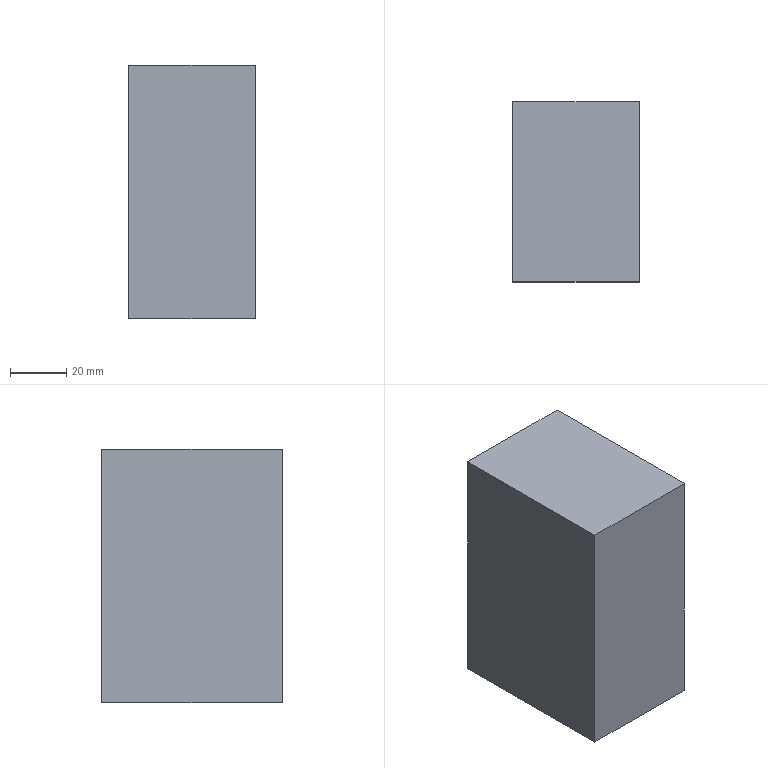Part | SolidWorks | features Extrusion 1 | 1 solid | 6 faces | box 45 x 64 x 90 mm | volume 259200 mm3 | plane 6
STEP:
#1=CARTESIAN_POINT('',(22.5,0.,45.));
#2=VERTEX_POINT('',#1);
#3=CARTESIAN_POINT('',(22.5,0.,-45.));
#4=VERTEX_POINT('',#3);
#5=CARTESIAN_POINT('',(22.5,0.,45.));
#6=DIRECTION('',(0.,0.,-1.));
#7=VECTOR('',#6,1000.);
#8=LINE('',#5,#7);
#9=EDGE_CURVE('',#2,#4,#8,.T.);
#10=ORIENTED_EDGE('',*,*,#9,.T.);
#11=CARTESIAN_POINT('',(22.5,64.,-45.));
#12=VERTEX_POINT('',#11);
#13=CARTESIAN_POINT('',(22.5,64.,-45.));
#14=DIRECTION('',(0.,-1.,0.));
#15=VECTOR('',#14,1000.);
#16=LINE('',#13,#15);
#17=EDGE_CURVE('',#12,#4,#16,.T.);
#18=ORIENTED_EDGE('',*,*,#17,.F.);
#19=CARTESIAN_POINT('',(22.5,64.,45.));
#20=VERTEX_POINT('',#19);
#21=CARTESIAN_POINT('',(22.5,64.,45.));
#22=DIRECTION('',(0.,0.,-1.));
#23=VECTOR('',#22,1000.);
#24=LINE('',#21,#23);
#25=EDGE_CURVE('',#20,#12,#24,.T.);
#26=ORIENTED_EDGE('',*,*,#25,.F.);
#27=CARTESIAN_POINT('',(22.5,64.,45.));
#28=DIRECTION('',(0.,-1.,0.));
#29=VECTOR('',#28,1000.);
#30=LINE('',#27,#29);
#31=EDGE_CURVE('',#20,#2,#30,.T.);
#32=ORIENTED_EDGE('',*,*,#31,.T.);
#33=EDGE_LOOP('',(#10,#18,#26,#32));
#34=FACE_OUTER_BOUND('',#33,.T.);
#35=CARTESIAN_POINT('',(22.5,64.,45.));
#36=DIRECTION('',(-1.,0.,0.));
#37=DIRECTION('',(0.,0.,1.));
#38=AXIS2_PLACEMENT_3D('',#35,#36,#37);
#39=PLANE('',#38);
#40=ADVANCED_FACE('',(#34),#39,.F.);
#41=CARTESIAN_POINT('',(-22.5,0.,-45.));
#42=VERTEX_POINT('',#41);
#43=CARTESIAN_POINT('',(-22.5,0.,-45.));
#44=DIRECTION('',(-1.,0.,0.));
#45=VECTOR('',#44,1000.);
#46=LINE('',#43,#45);
#47=EDGE_CURVE('',#4,#42,#46,.T.);
#48=ORIENTED_EDGE('',*,*,#47,.T.);
#49=CARTESIAN_POINT('',(-22.5,64.,-45.));
#50=VERTEX_POINT('',#49);
#51=CARTESIAN_POINT('',(-22.5,64.,-45.));
#52=DIRECTION('',(0.,-1.,0.));
#53=VECTOR('',#52,1000.);
#54=LINE('',#51,#53);
#55=EDGE_CURVE('',#50,#42,#54,.T.);
#56=ORIENTED_EDGE('',*,*,#55,.F.);
#57=CARTESIAN_POINT('',(-22.5,64.,-45.));
#58=DIRECTION('',(-1.,0.,0.));
#59=VECTOR('',#58,1000.);
#60=LINE('',#57,#59);
#61=EDGE_CURVE('',#12,#50,#60,.T.);
#62=ORIENTED_EDGE('',*,*,#61,.F.);
#63=ORIENTED_EDGE('',*,*,#17,.T.);
#64=EDGE_LOOP('',(#48,#56,#62,#63));
#65=FACE_OUTER_BOUND('',#64,.T.);
#66=CARTESIAN_POINT('',(-22.5,64.,-45.));
#67=DIRECTION('',(0.,0.,1.));
#68=DIRECTION('',(1.,0.,0.));
#69=AXIS2_PLACEMENT_3D('',#66,#67,#68);
#70=PLANE('',#69);
#71=ADVANCED_FACE('',(#65),#70,.F.);
#72=CARTESIAN_POINT('',(-22.5,0.,45.));
#73=VERTEX_POINT('',#72);
#74=CARTESIAN_POINT('',(-22.5,0.,45.));
#75=DIRECTION('',(0.,0.,1.));
#76=VECTOR('',#75,1000.);
#77=LINE('',#74,#76);
#78=EDGE_CURVE('',#42,#73,#77,.T.);
#79=ORIENTED_EDGE('',*,*,#78,.T.);
#80=CARTESIAN_POINT('',(-22.5,64.,45.));
#81=VERTEX_POINT('',#80);
#82=CARTESIAN_POINT('',(-22.5,64.,45.));
#83=DIRECTION('',(0.,-1.,0.));
#84=VECTOR('',#83,1000.);
#85=LINE('',#82,#84);
#86=EDGE_CURVE('',#81,#73,#85,.T.);
#87=ORIENTED_EDGE('',*,*,#86,.F.);
#88=CARTESIAN_POINT('',(-22.5,64.,45.));
#89=DIRECTION('',(0.,0.,1.));
#90=VECTOR('',#89,1000.);
#91=LINE('',#88,#90);
#92=EDGE_CURVE('',#50,#81,#91,.T.);
#93=ORIENTED_EDGE('',*,*,#92,.F.);
#94=ORIENTED_EDGE('',*,*,#55,.T.);
#95=EDGE_LOOP('',(#79,#87,#93,#94));
#96=FACE_OUTER_BOUND('',#95,.T.);
#97=CARTESIAN_POINT('',(-22.5,64.,45.));
#98=DIRECTION('',(1.,0.,0.));
#99=DIRECTION('',(0.,0.,-1.));
#100=AXIS2_PLACEMENT_3D('',#97,#98,#99);
#101=PLANE('',#100);
#102=ADVANCED_FACE('',(#96),#101,.F.);
#103=CARTESIAN_POINT('',(-22.5,0.,45.));
#104=DIRECTION('',(1.,0.,0.));
#105=VECTOR('',#104,1000.);
#106=LINE('',#103,#105);
#107=EDGE_CURVE('',#73,#2,#106,.T.);
#108=ORIENTED_EDGE('',*,*,#107,.T.);
#109=ORIENTED_EDGE('',*,*,#31,.F.);
#110=CARTESIAN_POINT('',(-22.5,64.,45.));
#111=DIRECTION('',(1.,0.,0.));
#112=VECTOR('',#111,1000.);
#113=LINE('',#110,#112);
#114=EDGE_CURVE('',#81,#20,#113,.T.);
#115=ORIENTED_EDGE('',*,*,#114,.F.);
#116=ORIENTED_EDGE('',*,*,#86,.T.);
#117=EDGE_LOOP('',(#108,#109,#115,#116));
#118=FACE_OUTER_BOUND('',#117,.T.);
#119=CARTESIAN_POINT('',(-22.5,64.,45.));
#120=DIRECTION('',(0.,0.,-1.));
#121=DIRECTION('',(-1.,0.,0.));
#122=AXIS2_PLACEMENT_3D('',#119,#120,#121);
#123=PLANE('',#122);
#124=ADVANCED_FACE('',(#118),#123,.F.);
#125=ORIENTED_EDGE('',*,*,#25,.T.);
#126=ORIENTED_EDGE('',*,*,#61,.T.);
#127=ORIENTED_EDGE('',*,*,#92,.T.);
#128=ORIENTED_EDGE('',*,*,#114,.T.);
#129=EDGE_LOOP('',(#125,#126,#127,#128));
#130=FACE_OUTER_BOUND('',#129,.T.);
#131=CARTESIAN_POINT('',(0.,64.,0.));
#132=DIRECTION('',(0.,-1.,0.));
#133=DIRECTION('',(0.,0.,-1.));
#134=AXIS2_PLACEMENT_3D('',#131,#132,#133);
#135=PLANE('',#134);
#136=ADVANCED_FACE('',(#130),#135,.F.);
#137=ORIENTED_EDGE('',*,*,#9,.F.);
#138=ORIENTED_EDGE('',*,*,#107,.F.);
#139=ORIENTED_EDGE('',*,*,#78,.F.);
#140=ORIENTED_EDGE('',*,*,#47,.F.);
#141=EDGE_LOOP('',(#137,#138,#139,#140));
#142=FACE_OUTER_BOUND('',#141,.T.);
#143=CARTESIAN_POINT('',(0.,0.,0.));
#144=DIRECTION('',(0.,-1.,0.));
#145=DIRECTION('',(0.,0.,-1.));
#146=AXIS2_PLACEMENT_3D('',#143,#144,#145);
#147=PLANE('',#146);
#148=ADVANCED_FACE('',(#142),#147,.T.);
#149=CLOSED_SHELL('',(#40,#71,#102,#124,#136,#148));
#150=MANIFOLD_SOLID_BREP('',#149);
#151=CARTESIAN_POINT('',(0.,0.,0.));
#152=DIRECTION('',(0.,0.,1.));
#153=DIRECTION('',(1.,0.,0.));
#154=AXIS2_PLACEMENT_3D('',#151,#152,#153);
#155=(LENGTH_UNIT()NAMED_UNIT(*)SI_UNIT(.MILLI.,.METRE.));
#156=UNCERTAINTY_MEASURE_WITH_UNIT(LENGTH_MEASURE(0.00001),#155,'','');
#157=(NAMED_UNIT(*)PLANE_ANGLE_UNIT()SI_UNIT($,.RADIAN.));
#158=(NAMED_UNIT(*)SI_UNIT($,.STERADIAN.)SOLID_ANGLE_UNIT());
#159=(GEOMETRIC_REPRESENTATION_CONTEXT(3)GLOBAL_UNCERTAINTY_ASSIGNED_CONTEXT((#156))GLOBAL_UNIT_ASSIGNED_CONTEXT((#155,#157,#158))REPRESENTATION_CONTEXT('',''));
#160=ADVANCED_BREP_SHAPE_REPRESENTATION('',(#150,#154),#159);